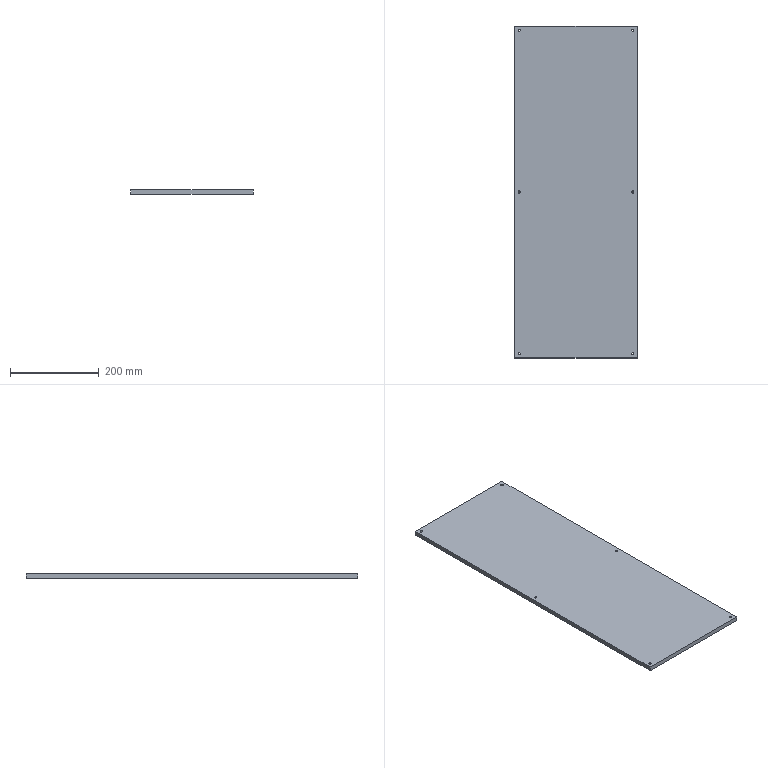Part | STEP file | SynoNew-0304-061 | 1 solid | 12 faces | box 277 x 750 x 10 mm | volume 2076322 mm3 | cylinder 6 | plane 6 | commonest cylinder face diameters 5 x6
STEP:
#1=CARTESIAN_POINT('',(131.,-365.,10.));
#2=VERTEX_POINT('',#1);
#3=CARTESIAN_POINT('',(126.,-365.,10.));
#4=VERTEX_POINT('',#3);
#5=CARTESIAN_POINT('',(128.5,-365.,10.));
#6=DIRECTION('',(0.,0.,-1.));
#7=DIRECTION('',(1.,0.,0.));
#8=AXIS2_PLACEMENT_3D('',#5,#6,#7);
#9=CIRCLE('',#8,2.5);
#10=EDGE_CURVE('',#2,#4,#9,.T.);
#11=ORIENTED_EDGE('',*,*,#10,.F.);
#12=CARTESIAN_POINT('',(128.5,-365.,10.));
#13=DIRECTION('',(0.,0.,-1.));
#14=DIRECTION('',(1.,0.,0.));
#15=AXIS2_PLACEMENT_3D('',#12,#13,#14);
#16=CIRCLE('',#15,2.5);
#17=EDGE_CURVE('',#4,#2,#16,.T.);
#18=ORIENTED_EDGE('',*,*,#17,.F.);
#19=CARTESIAN_POINT('',(126.,-365.,0.));
#20=VERTEX_POINT('',#19);
#21=CARTESIAN_POINT('',(126.,-365.,-789.581));
#22=DIRECTION('',(0.,0.,-1.));
#23=VECTOR('',#22,2.5);
#24=LINE('',#21,#23);
#25=EDGE_CURVE('',#4,#20,#24,.T.);
#26=ORIENTED_EDGE('',*,*,#25,.T.);
#27=CARTESIAN_POINT('',(128.5,-365.,0.));
#28=DIRECTION('',(0.,0.,1.));
#29=DIRECTION('',(1.,0.,0.));
#30=AXIS2_PLACEMENT_3D('',#27,#28,#29);
#31=CIRCLE('',#30,2.5);
#32=EDGE_CURVE('',#20,#20,#31,.T.);
#33=ORIENTED_EDGE('',*,*,#32,.F.);
#34=ORIENTED_EDGE('',*,*,#25,.F.);
#35=EDGE_LOOP('',(#11,#18,#26,#33,#34));
#36=FACE_OUTER_BOUND('',#35,.T.);
#37=CARTESIAN_POINT('',(128.5,-365.,-789.581));
#38=DIRECTION('',(0.,0.,1.));
#39=DIRECTION('',(1.,0.,0.));
#40=AXIS2_PLACEMENT_3D('',#37,#38,#39);
#41=CYLINDRICAL_SURFACE('',#40,2.5);
#42=ADVANCED_FACE('',(#36),#41,.F.);
#43=CARTESIAN_POINT('',(131.,365.,10.));
#44=VERTEX_POINT('',#43);
#45=CARTESIAN_POINT('',(126.,365.,10.));
#46=VERTEX_POINT('',#45);
#47=CARTESIAN_POINT('',(128.5,365.,10.));
#48=DIRECTION('',(0.,0.,-1.));
#49=DIRECTION('',(1.,0.,0.));
#50=AXIS2_PLACEMENT_3D('',#47,#48,#49);
#51=CIRCLE('',#50,2.5);
#52=EDGE_CURVE('',#44,#46,#51,.T.);
#53=ORIENTED_EDGE('',*,*,#52,.F.);
#54=CARTESIAN_POINT('',(128.5,365.,10.));
#55=DIRECTION('',(0.,0.,-1.));
#56=DIRECTION('',(1.,0.,0.));
#57=AXIS2_PLACEMENT_3D('',#54,#55,#56);
#58=CIRCLE('',#57,2.5);
#59=EDGE_CURVE('',#46,#44,#58,.T.);
#60=ORIENTED_EDGE('',*,*,#59,.F.);
#61=CARTESIAN_POINT('',(126.,365.,0.));
#62=VERTEX_POINT('',#61);
#63=CARTESIAN_POINT('',(126.,365.,-789.581));
#64=DIRECTION('',(0.,0.,-1.));
#65=VECTOR('',#64,2.5);
#66=LINE('',#63,#65);
#67=EDGE_CURVE('',#46,#62,#66,.T.);
#68=ORIENTED_EDGE('',*,*,#67,.T.);
#69=CARTESIAN_POINT('',(128.5,365.,0.));
#70=DIRECTION('',(0.,0.,1.));
#71=DIRECTION('',(1.,0.,0.));
#72=AXIS2_PLACEMENT_3D('',#69,#70,#71);
#73=CIRCLE('',#72,2.5);
#74=EDGE_CURVE('',#62,#62,#73,.T.);
#75=ORIENTED_EDGE('',*,*,#74,.F.);
#76=ORIENTED_EDGE('',*,*,#67,.F.);
#77=EDGE_LOOP('',(#53,#60,#68,#75,#76));
#78=FACE_OUTER_BOUND('',#77,.T.);
#79=CARTESIAN_POINT('',(128.5,365.,-789.581));
#80=DIRECTION('',(0.,0.,1.));
#81=DIRECTION('',(1.,0.,0.));
#82=AXIS2_PLACEMENT_3D('',#79,#80,#81);
#83=CYLINDRICAL_SURFACE('',#82,2.5);
#84=ADVANCED_FACE('',(#78),#83,.F.);
#85=CARTESIAN_POINT('',(-126.,0.,10.));
#86=VERTEX_POINT('',#85);
#87=CARTESIAN_POINT('',(-131.,0.,10.));
#88=VERTEX_POINT('',#87);
#89=CARTESIAN_POINT('',(-128.5,0.,10.));
#90=DIRECTION('',(0.,0.,-1.));
#91=DIRECTION('',(1.,0.,0.));
#92=AXIS2_PLACEMENT_3D('',#89,#90,#91);
#93=CIRCLE('',#92,2.5);
#94=EDGE_CURVE('',#86,#88,#93,.T.);
#95=ORIENTED_EDGE('',*,*,#94,.F.);
#96=CARTESIAN_POINT('',(-128.5,0.,10.));
#97=DIRECTION('',(0.,0.,-1.));
#98=DIRECTION('',(1.,0.,0.));
#99=AXIS2_PLACEMENT_3D('',#96,#97,#98);
#100=CIRCLE('',#99,2.5);
#101=EDGE_CURVE('',#88,#86,#100,.T.);
#102=ORIENTED_EDGE('',*,*,#101,.F.);
#103=CARTESIAN_POINT('',(-131.,0.,0.));
#104=VERTEX_POINT('',#103);
#105=CARTESIAN_POINT('',(-131.,0.,-789.581));
#106=DIRECTION('',(0.,0.,-1.));
#107=VECTOR('',#106,2.5);
#108=LINE('',#105,#107);
#109=EDGE_CURVE('',#88,#104,#108,.T.);
#110=ORIENTED_EDGE('',*,*,#109,.T.);
#111=CARTESIAN_POINT('',(-128.5,0.,0.));
#112=DIRECTION('',(0.,0.,1.));
#113=DIRECTION('',(1.,0.,0.));
#114=AXIS2_PLACEMENT_3D('',#111,#112,#113);
#115=CIRCLE('',#114,2.5);
#116=EDGE_CURVE('',#104,#104,#115,.T.);
#117=ORIENTED_EDGE('',*,*,#116,.F.);
#118=ORIENTED_EDGE('',*,*,#109,.F.);
#119=EDGE_LOOP('',(#95,#102,#110,#117,#118));
#120=FACE_OUTER_BOUND('',#119,.T.);
#121=CARTESIAN_POINT('',(-128.5,0.,-789.581));
#122=DIRECTION('',(0.,0.,1.));
#123=DIRECTION('',(1.,0.,0.));
#124=AXIS2_PLACEMENT_3D('',#121,#122,#123);
#125=CYLINDRICAL_SURFACE('',#124,2.5);
#126=ADVANCED_FACE('',(#120),#125,.F.);
#127=CARTESIAN_POINT('',(131.,0.,10.));
#128=VERTEX_POINT('',#127);
#129=CARTESIAN_POINT('',(126.,0.,10.));
#130=VERTEX_POINT('',#129);
#131=CARTESIAN_POINT('',(128.5,0.,10.));
#132=DIRECTION('',(0.,0.,-1.));
#133=DIRECTION('',(1.,0.,0.));
#134=AXIS2_PLACEMENT_3D('',#131,#132,#133);
#135=CIRCLE('',#134,2.5);
#136=EDGE_CURVE('',#128,#130,#135,.T.);
#137=ORIENTED_EDGE('',*,*,#136,.F.);
#138=CARTESIAN_POINT('',(128.5,0.,10.));
#139=DIRECTION('',(0.,0.,-1.));
#140=DIRECTION('',(1.,0.,0.));
#141=AXIS2_PLACEMENT_3D('',#138,#139,#140);
#142=CIRCLE('',#141,2.5);
#143=EDGE_CURVE('',#130,#128,#142,.T.);
#144=ORIENTED_EDGE('',*,*,#143,.F.);
#145=CARTESIAN_POINT('',(126.,0.,0.));
#146=VERTEX_POINT('',#145);
#147=CARTESIAN_POINT('',(126.,0.,-789.581));
#148=DIRECTION('',(0.,0.,-1.));
#149=VECTOR('',#148,2.5);
#150=LINE('',#147,#149);
#151=EDGE_CURVE('',#130,#146,#150,.T.);
#152=ORIENTED_EDGE('',*,*,#151,.T.);
#153=CARTESIAN_POINT('',(128.5,0.,0.));
#154=DIRECTION('',(0.,0.,1.));
#155=DIRECTION('',(1.,0.,0.));
#156=AXIS2_PLACEMENT_3D('',#153,#154,#155);
#157=CIRCLE('',#156,2.5);
#158=EDGE_CURVE('',#146,#146,#157,.T.);
#159=ORIENTED_EDGE('',*,*,#158,.F.);
#160=ORIENTED_EDGE('',*,*,#151,.F.);
#161=EDGE_LOOP('',(#137,#144,#152,#159,#160));
#162=FACE_OUTER_BOUND('',#161,.T.);
#163=CARTESIAN_POINT('',(128.5,0.,-789.581));
#164=DIRECTION('',(0.,0.,1.));
#165=DIRECTION('',(1.,0.,0.));
#166=AXIS2_PLACEMENT_3D('',#163,#164,#165);
#167=CYLINDRICAL_SURFACE('',#166,2.5);
#168=ADVANCED_FACE('',(#162),#167,.F.);
#169=CARTESIAN_POINT('',(-126.,365.,10.));
#170=VERTEX_POINT('',#169);
#171=CARTESIAN_POINT('',(-131.,365.,10.));
#172=VERTEX_POINT('',#171);
#173=CARTESIAN_POINT('',(-128.5,365.,10.));
#174=DIRECTION('',(0.,0.,-1.));
#175=DIRECTION('',(1.,0.,0.));
#176=AXIS2_PLACEMENT_3D('',#173,#174,#175);
#177=CIRCLE('',#176,2.5);
#178=EDGE_CURVE('',#170,#172,#177,.T.);
#179=ORIENTED_EDGE('',*,*,#178,.F.);
#180=CARTESIAN_POINT('',(-128.5,365.,10.));
#181=DIRECTION('',(0.,0.,-1.));
#182=DIRECTION('',(1.,0.,0.));
#183=AXIS2_PLACEMENT_3D('',#180,#181,#182);
#184=CIRCLE('',#183,2.5);
#185=EDGE_CURVE('',#172,#170,#184,.T.);
#186=ORIENTED_EDGE('',*,*,#185,.F.);
#187=CARTESIAN_POINT('',(-131.,365.,0.));
#188=VERTEX_POINT('',#187);
#189=CARTESIAN_POINT('',(-131.,365.,-789.581));
#190=DIRECTION('',(0.,0.,-1.));
#191=VECTOR('',#190,2.5);
#192=LINE('',#189,#191);
#193=EDGE_CURVE('',#172,#188,#192,.T.);
#194=ORIENTED_EDGE('',*,*,#193,.T.);
#195=CARTESIAN_POINT('',(-128.5,365.,0.));
#196=DIRECTION('',(0.,0.,1.));
#197=DIRECTION('',(1.,0.,0.));
#198=AXIS2_PLACEMENT_3D('',#195,#196,#197);
#199=CIRCLE('',#198,2.5);
#200=EDGE_CURVE('',#188,#188,#199,.T.);
#201=ORIENTED_EDGE('',*,*,#200,.F.);
#202=ORIENTED_EDGE('',*,*,#193,.F.);
#203=EDGE_LOOP('',(#179,#186,#194,#201,#202));
#204=FACE_OUTER_BOUND('',#203,.T.);
#205=CARTESIAN_POINT('',(-128.5,365.,-789.581));
#206=DIRECTION('',(0.,0.,1.));
#207=DIRECTION('',(1.,0.,0.));
#208=AXIS2_PLACEMENT_3D('',#205,#206,#207);
#209=CYLINDRICAL_SURFACE('',#208,2.5);
#210=ADVANCED_FACE('',(#204),#209,.F.);
#211=CARTESIAN_POINT('',(-126.,-365.,10.));
#212=VERTEX_POINT('',#211);
#213=CARTESIAN_POINT('',(-131.,-365.,10.));
#214=VERTEX_POINT('',#213);
#215=CARTESIAN_POINT('',(-128.5,-365.,10.));
#216=DIRECTION('',(0.,0.,-1.));
#217=DIRECTION('',(1.,0.,0.));
#218=AXIS2_PLACEMENT_3D('',#215,#216,#217);
#219=CIRCLE('',#218,2.5);
#220=EDGE_CURVE('',#212,#214,#219,.T.);
#221=ORIENTED_EDGE('',*,*,#220,.F.);
#222=CARTESIAN_POINT('',(-128.5,-365.,10.));
#223=DIRECTION('',(0.,0.,-1.));
#224=DIRECTION('',(1.,0.,0.));
#225=AXIS2_PLACEMENT_3D('',#222,#223,#224);
#226=CIRCLE('',#225,2.5);
#227=EDGE_CURVE('',#214,#212,#226,.T.);
#228=ORIENTED_EDGE('',*,*,#227,.F.);
#229=CARTESIAN_POINT('',(-131.,-365.,0.));
#230=VERTEX_POINT('',#229);
#231=CARTESIAN_POINT('',(-131.,-365.,-789.581));
#232=DIRECTION('',(0.,0.,-1.));
#233=VECTOR('',#232,2.5);
#234=LINE('',#231,#233);
#235=EDGE_CURVE('',#214,#230,#234,.T.);
#236=ORIENTED_EDGE('',*,*,#235,.T.);
#237=CARTESIAN_POINT('',(-128.5,-365.,0.));
#238=DIRECTION('',(0.,0.,1.));
#239=DIRECTION('',(1.,0.,0.));
#240=AXIS2_PLACEMENT_3D('',#237,#238,#239);
#241=CIRCLE('',#240,2.5);
#242=EDGE_CURVE('',#230,#230,#241,.T.);
#243=ORIENTED_EDGE('',*,*,#242,.F.);
#244=ORIENTED_EDGE('',*,*,#235,.F.);
#245=EDGE_LOOP('',(#221,#228,#236,#243,#244));
#246=FACE_OUTER_BOUND('',#245,.T.);
#247=CARTESIAN_POINT('',(-128.5,-365.,-789.581));
#248=DIRECTION('',(0.,0.,1.));
#249=DIRECTION('',(1.,0.,0.));
#250=AXIS2_PLACEMENT_3D('',#247,#248,#249);
#251=CYLINDRICAL_SURFACE('',#250,2.5);
#252=ADVANCED_FACE('',(#246),#251,.F.);
#253=CARTESIAN_POINT('',(-138.5,-375.,0.));
#254=VERTEX_POINT('',#253);
#255=CARTESIAN_POINT('',(138.5,-375.,0.));
#256=VERTEX_POINT('',#255);
#257=CARTESIAN_POINT('',(-138.5,-375.,0.));
#258=DIRECTION('',(1.,0.,0.));
#259=VECTOR('',#258,10.);
#260=LINE('',#257,#259);
#261=EDGE_CURVE('',#254,#256,#260,.T.);
#262=ORIENTED_EDGE('',*,*,#261,.T.);
#263=CARTESIAN_POINT('',(138.5,-375.,10.));
#264=VERTEX_POINT('',#263);
#265=CARTESIAN_POINT('',(138.5,-375.,0.));
#266=DIRECTION('',(0.,0.,1.));
#267=VECTOR('',#266,10.);
#268=LINE('',#265,#267);
#269=EDGE_CURVE('',#256,#264,#268,.T.);
#270=ORIENTED_EDGE('',*,*,#269,.T.);
#271=CARTESIAN_POINT('',(-138.5,-375.,10.));
#272=VERTEX_POINT('',#271);
#273=CARTESIAN_POINT('',(-138.5,-375.,10.));
#274=DIRECTION('',(1.,0.,0.));
#275=VECTOR('',#274,10.);
#276=LINE('',#273,#275);
#277=EDGE_CURVE('',#272,#264,#276,.T.);
#278=ORIENTED_EDGE('',*,*,#277,.F.);
#279=CARTESIAN_POINT('',(-138.5,-375.,0.));
#280=DIRECTION('',(0.,0.,1.));
#281=VECTOR('',#280,10.);
#282=LINE('',#279,#281);
#283=EDGE_CURVE('',#254,#272,#282,.T.);
#284=ORIENTED_EDGE('',*,*,#283,.F.);
#285=EDGE_LOOP('',(#262,#270,#278,#284));
#286=FACE_OUTER_BOUND('',#285,.T.);
#287=CARTESIAN_POINT('',(-138.5,-375.,0.));
#288=DIRECTION('',(0.,-1.,0.));
#289=DIRECTION('',(1.,0.,0.));
#290=AXIS2_PLACEMENT_3D('',#287,#288,#289);
#291=PLANE('',#290);
#292=ADVANCED_FACE('',(#286),#291,.T.);
#293=CARTESIAN_POINT('',(-138.5,375.,0.));
#294=VERTEX_POINT('',#293);
#295=CARTESIAN_POINT('',(-138.5,375.,0.));
#296=DIRECTION('',(0.,-1.,0.));
#297=VECTOR('',#296,10.);
#298=LINE('',#295,#297);
#299=EDGE_CURVE('',#294,#254,#298,.T.);
#300=ORIENTED_EDGE('',*,*,#299,.T.);
#301=ORIENTED_EDGE('',*,*,#283,.T.);
#302=CARTESIAN_POINT('',(-138.5,375.,10.));
#303=VERTEX_POINT('',#302);
#304=CARTESIAN_POINT('',(-138.5,375.,10.));
#305=DIRECTION('',(0.,-1.,0.));
#306=VECTOR('',#305,10.);
#307=LINE('',#304,#306);
#308=EDGE_CURVE('',#303,#272,#307,.T.);
#309=ORIENTED_EDGE('',*,*,#308,.F.);
#310=CARTESIAN_POINT('',(-138.5,375.,0.));
#311=DIRECTION('',(0.,0.,1.));
#312=VECTOR('',#311,10.);
#313=LINE('',#310,#312);
#314=EDGE_CURVE('',#294,#303,#313,.T.);
#315=ORIENTED_EDGE('',*,*,#314,.F.);
#316=EDGE_LOOP('',(#300,#301,#309,#315));
#317=FACE_OUTER_BOUND('',#316,.T.);
#318=CARTESIAN_POINT('',(-138.5,375.,0.));
#319=DIRECTION('',(-1.,0.,0.));
#320=DIRECTION('',(0.,-1.,0.));
#321=AXIS2_PLACEMENT_3D('',#318,#319,#320);
#322=PLANE('',#321);
#323=ADVANCED_FACE('',(#317),#322,.T.);
#324=CARTESIAN_POINT('',(138.5,375.,0.));
#325=VERTEX_POINT('',#324);
#326=CARTESIAN_POINT('',(138.5,375.,0.));
#327=DIRECTION('',(-1.,0.,0.));
#328=VECTOR('',#327,10.);
#329=LINE('',#326,#328);
#330=EDGE_CURVE('',#325,#294,#329,.T.);
#331=ORIENTED_EDGE('',*,*,#330,.T.);
#332=ORIENTED_EDGE('',*,*,#314,.T.);
#333=CARTESIAN_POINT('',(138.5,375.,10.));
#334=VERTEX_POINT('',#333);
#335=CARTESIAN_POINT('',(138.5,375.,10.));
#336=DIRECTION('',(-1.,0.,0.));
#337=VECTOR('',#336,10.);
#338=LINE('',#335,#337);
#339=EDGE_CURVE('',#334,#303,#338,.T.);
#340=ORIENTED_EDGE('',*,*,#339,.F.);
#341=CARTESIAN_POINT('',(138.5,375.,0.));
#342=DIRECTION('',(0.,0.,1.));
#343=VECTOR('',#342,10.);
#344=LINE('',#341,#343);
#345=EDGE_CURVE('',#325,#334,#344,.T.);
#346=ORIENTED_EDGE('',*,*,#345,.F.);
#347=EDGE_LOOP('',(#331,#332,#340,#346));
#348=FACE_OUTER_BOUND('',#347,.T.);
#349=CARTESIAN_POINT('',(138.5,375.,0.));
#350=DIRECTION('',(0.,1.,0.));
#351=DIRECTION('',(-1.,0.,0.));
#352=AXIS2_PLACEMENT_3D('',#349,#350,#351);
#353=PLANE('',#352);
#354=ADVANCED_FACE('',(#348),#353,.T.);
#355=CARTESIAN_POINT('',(138.5,-375.,0.));
#356=DIRECTION('',(0.,1.,0.));
#357=VECTOR('',#356,10.);
#358=LINE('',#355,#357);
#359=EDGE_CURVE('',#256,#325,#358,.T.);
#360=ORIENTED_EDGE('',*,*,#359,.T.);
#361=ORIENTED_EDGE('',*,*,#345,.T.);
#362=CARTESIAN_POINT('',(138.5,-375.,10.));
#363=DIRECTION('',(0.,1.,0.));
#364=VECTOR('',#363,10.);
#365=LINE('',#362,#364);
#366=EDGE_CURVE('',#264,#334,#365,.T.);
#367=ORIENTED_EDGE('',*,*,#366,.F.);
#368=ORIENTED_EDGE('',*,*,#269,.F.);
#369=EDGE_LOOP('',(#360,#361,#367,#368));
#370=FACE_OUTER_BOUND('',#369,.T.);
#371=CARTESIAN_POINT('',(138.5,-375.,0.));
#372=DIRECTION('',(1.,0.,0.));
#373=DIRECTION('',(0.,1.,0.));
#374=AXIS2_PLACEMENT_3D('',#371,#372,#373);
#375=PLANE('',#374);
#376=ADVANCED_FACE('',(#370),#375,.T.);
#377=ORIENTED_EDGE('',*,*,#366,.T.);
#378=ORIENTED_EDGE('',*,*,#339,.T.);
#379=ORIENTED_EDGE('',*,*,#308,.T.);
#380=ORIENTED_EDGE('',*,*,#277,.T.);
#381=EDGE_LOOP('',(#377,#378,#379,#380));
#382=FACE_OUTER_BOUND('',#381,.T.);
#383=ORIENTED_EDGE('',*,*,#10,.T.);
#384=ORIENTED_EDGE('',*,*,#17,.T.);
#385=EDGE_LOOP('',(#383,#384));
#386=FACE_BOUND('',#385,.T.);
#387=ORIENTED_EDGE('',*,*,#52,.T.);
#388=ORIENTED_EDGE('',*,*,#59,.T.);
#389=EDGE_LOOP('',(#387,#388));
#390=FACE_BOUND('',#389,.T.);
#391=ORIENTED_EDGE('',*,*,#94,.T.);
#392=ORIENTED_EDGE('',*,*,#101,.T.);
#393=EDGE_LOOP('',(#391,#392));
#394=FACE_BOUND('',#393,.T.);
#395=ORIENTED_EDGE('',*,*,#136,.T.);
#396=ORIENTED_EDGE('',*,*,#143,.T.);
#397=EDGE_LOOP('',(#395,#396));
#398=FACE_BOUND('',#397,.T.);
#399=ORIENTED_EDGE('',*,*,#178,.T.);
#400=ORIENTED_EDGE('',*,*,#185,.T.);
#401=EDGE_LOOP('',(#399,#400));
#402=FACE_BOUND('',#401,.T.);
#403=ORIENTED_EDGE('',*,*,#220,.T.);
#404=ORIENTED_EDGE('',*,*,#227,.T.);
#405=EDGE_LOOP('',(#403,#404));
#406=FACE_BOUND('',#405,.T.);
#407=CARTESIAN_POINT('',(0.,0.,10.));
#408=DIRECTION('',(0.,0.,1.));
#409=DIRECTION('',(1.,0.,0.));
#410=AXIS2_PLACEMENT_3D('',#407,#408,#409);
#411=PLANE('',#410);
#412=ADVANCED_FACE('',(#382,#386,#390,#394,#398,#402,#406),#411,.T.);
#413=ORIENTED_EDGE('',*,*,#359,.F.);
#414=ORIENTED_EDGE('',*,*,#261,.F.);
#415=ORIENTED_EDGE('',*,*,#299,.F.);
#416=ORIENTED_EDGE('',*,*,#330,.F.);
#417=EDGE_LOOP('',(#413,#414,#415,#416));
#418=FACE_OUTER_BOUND('',#417,.T.);
#419=ORIENTED_EDGE('',*,*,#32,.T.);
#420=EDGE_LOOP('',(#419));
#421=FACE_BOUND('',#420,.T.);
#422=ORIENTED_EDGE('',*,*,#74,.T.);
#423=EDGE_LOOP('',(#422));
#424=FACE_BOUND('',#423,.T.);
#425=ORIENTED_EDGE('',*,*,#116,.T.);
#426=EDGE_LOOP('',(#425));
#427=FACE_BOUND('',#426,.T.);
#428=ORIENTED_EDGE('',*,*,#158,.T.);
#429=EDGE_LOOP('',(#428));
#430=FACE_BOUND('',#429,.T.);
#431=ORIENTED_EDGE('',*,*,#200,.T.);
#432=EDGE_LOOP('',(#431));
#433=FACE_BOUND('',#432,.T.);
#434=ORIENTED_EDGE('',*,*,#242,.T.);
#435=EDGE_LOOP('',(#434));
#436=FACE_BOUND('',#435,.T.);
#437=CARTESIAN_POINT('',(0.,0.,0.));
#438=DIRECTION('',(0.,0.,1.));
#439=DIRECTION('',(1.,0.,0.));
#440=AXIS2_PLACEMENT_3D('',#437,#438,#439);
#441=PLANE('',#440);
#442=ADVANCED_FACE('',(#418,#421,#424,#427,#430,#433,#436),#441,.F.);
#443=CLOSED_SHELL('',(#42,#84,#126,#168,#210,#252,#292,#323,#354,#376,#412,#442));
#444=MANIFOLD_SOLID_BREP('',#443);
#445=(LENGTH_UNIT()NAMED_UNIT(*)SI_UNIT(.MILLI.,.METRE.));
#446=UNCERTAINTY_MEASURE_WITH_UNIT(LENGTH_MEASURE(0.01),#445,'','');
#447=(NAMED_UNIT(*)PLANE_ANGLE_UNIT()SI_UNIT($,.RADIAN.));
#448=(NAMED_UNIT(*)SI_UNIT($,.STERADIAN.)SOLID_ANGLE_UNIT());
#449=(GEOMETRIC_REPRESENTATION_CONTEXT(3)GLOBAL_UNCERTAINTY_ASSIGNED_CONTEXT((#446))GLOBAL_UNIT_ASSIGNED_CONTEXT((#445,#447,#448))REPRESENTATION_CONTEXT('',''));
#450=ADVANCED_BREP_SHAPE_REPRESENTATION('',(#444),#449);